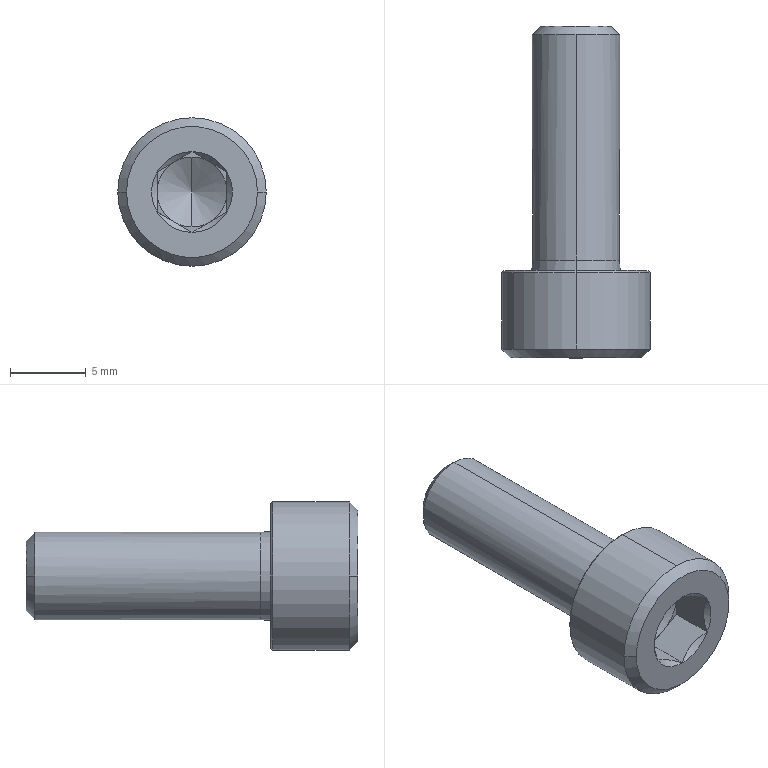Part | SolidWorks | features BaseBody 1 | 1 solid | 35 faces | box 9.808 x 21.923 x 9.808 mm | volume 789.355 mm3 | cone 16 | plane 15 | cylinder 4 | commonest cylinder face diameters 5.769 x2 9.808 x2
STEP:
#1=CARTESIAN_POINT('',(256.285,217.203,292.308));
#2=VERTEX_POINT('',#1);
#3=CARTESIAN_POINT('',(253.4,217.203,295.192));
#4=VERTEX_POINT('',#3);
#5=CARTESIAN_POINT('',(253.4,217.203,292.308));
#6=DIRECTION('',(0.,-1.,0.));
#7=DIRECTION('',(0.,0.,-1.));
#8=AXIS2_PLACEMENT_3D('',#5,#6,#7);
#9=CIRCLE('',#8,2.885);
#10=EDGE_CURVE('',#2,#4,#9,.T.);
#11=ORIENTED_EDGE('',*,*,#10,.T.);
#12=CARTESIAN_POINT('',(253.4,202.308,295.192));
#13=VERTEX_POINT('',#12);
#14=CARTESIAN_POINT('',(253.4,217.769,295.192));
#15=DIRECTION('',(0.,-1.,0.));
#16=VECTOR('',#15,1000.);
#17=LINE('',#14,#16);
#18=EDGE_CURVE('',#4,#13,#17,.T.);
#19=ORIENTED_EDGE('',*,*,#18,.T.);
#20=CARTESIAN_POINT('',(253.4,202.308,289.423));
#21=VERTEX_POINT('',#20);
#22=CARTESIAN_POINT('',(253.4,202.308,292.308));
#23=DIRECTION('',(0.,1.,0.));
#24=DIRECTION('',(0.,0.,-1.));
#25=AXIS2_PLACEMENT_3D('',#22,#23,#24);
#26=CIRCLE('',#25,2.885);
#27=EDGE_CURVE('',#13,#21,#26,.T.);
#28=ORIENTED_EDGE('',*,*,#27,.T.);
#29=CARTESIAN_POINT('',(253.4,217.203,289.423));
#30=VERTEX_POINT('',#29);
#31=CARTESIAN_POINT('',(253.4,217.769,289.423));
#32=DIRECTION('',(0.,-1.,0.));
#33=VECTOR('',#32,1000.);
#34=LINE('',#31,#33);
#35=EDGE_CURVE('',#30,#21,#34,.T.);
#36=ORIENTED_EDGE('',*,*,#35,.F.);
#37=CARTESIAN_POINT('',(253.4,217.203,292.308));
#38=DIRECTION('',(0.,-1.,0.));
#39=DIRECTION('',(0.,0.,-1.));
#40=AXIS2_PLACEMENT_3D('',#37,#38,#39);
#41=CIRCLE('',#40,2.885);
#42=EDGE_CURVE('',#30,#2,#41,.T.);
#43=ORIENTED_EDGE('',*,*,#42,.T.);
#44=EDGE_LOOP('',(#11,#19,#28,#36,#43));
#45=FACE_OUTER_BOUND('',#44,.T.);
#46=CARTESIAN_POINT('',(253.4,217.769,292.308));
#47=DIRECTION('',(0.,-1.,0.));
#48=DIRECTION('',(0.,0.,-1.));
#49=AXIS2_PLACEMENT_3D('',#46,#47,#48);
#50=CYLINDRICAL_SURFACE('',#49,2.885);
#51=ADVANCED_FACE('',(#45),#50,.T.);
#52=CARTESIAN_POINT('',(255.719,217.769,292.308));
#53=VERTEX_POINT('',#52);
#54=CARTESIAN_POINT('',(251.082,217.769,292.308));
#55=VERTEX_POINT('',#54);
#56=CARTESIAN_POINT('',(253.4,217.769,292.308));
#57=DIRECTION('',(0.,-1.,0.));
#58=DIRECTION('',(1.,0.,0.));
#59=AXIS2_PLACEMENT_3D('',#56,#57,#58);
#60=CIRCLE('',#59,2.319);
#61=EDGE_CURVE('',#53,#55,#60,.T.);
#62=ORIENTED_EDGE('',*,*,#61,.T.);
#63=CARTESIAN_POINT('',(250.516,217.203,292.308));
#64=VERTEX_POINT('',#63);
#65=CARTESIAN_POINT('',(250.516,217.203,292.308));
#66=DIRECTION('',(-0.7071,-0.7071,0.));
#67=VECTOR('',#66,1000.);
#68=LINE('',#65,#67);
#69=EDGE_CURVE('',#55,#64,#68,.T.);
#70=ORIENTED_EDGE('',*,*,#69,.T.);
#71=CARTESIAN_POINT('',(253.4,217.203,292.308));
#72=DIRECTION('',(0.,-1.,0.));
#73=DIRECTION('',(0.,0.,-1.));
#74=AXIS2_PLACEMENT_3D('',#71,#72,#73);
#75=CIRCLE('',#74,2.885);
#76=EDGE_CURVE('',#4,#64,#75,.T.);
#77=ORIENTED_EDGE('',*,*,#76,.F.);
#78=ORIENTED_EDGE('',*,*,#10,.F.);
#79=CARTESIAN_POINT('',(256.285,217.203,292.308));
#80=DIRECTION('',(0.7071,-0.7071,0.));
#81=VECTOR('',#80,1000.);
#82=LINE('',#79,#81);
#83=EDGE_CURVE('',#53,#2,#82,.T.);
#84=ORIENTED_EDGE('',*,*,#83,.F.);
#85=EDGE_LOOP('',(#62,#70,#77,#78,#84));
#86=FACE_OUTER_BOUND('',#85,.T.);
#87=CARTESIAN_POINT('',(253.4,217.203,292.308));
#88=DIRECTION('',(0.,-1.,0.));
#89=DIRECTION('',(1.,0.,0.));
#90=AXIS2_PLACEMENT_3D('',#87,#88,#89);
#91=CONICAL_SURFACE('',#90,2.885,0.7854);
#92=ADVANCED_FACE('',(#86),#91,.T.);
#93=ORIENTED_EDGE('',*,*,#27,.F.);
#94=CARTESIAN_POINT('',(253.4,201.615,295.25));
#95=VERTEX_POINT('',#94);
#96=CARTESIAN_POINT('',(253.4,201.615,295.25));
#97=DIRECTION('',(0.,-0.9965,0.08305));
#98=VECTOR('',#97,1000.);
#99=LINE('',#96,#98);
#100=EDGE_CURVE('',#13,#95,#99,.T.);
#101=ORIENTED_EDGE('',*,*,#100,.T.);
#102=CARTESIAN_POINT('',(253.4,201.615,289.365));
#103=VERTEX_POINT('',#102);
#104=CARTESIAN_POINT('',(253.4,201.615,292.308));
#105=DIRECTION('',(0.,1.,0.));
#106=DIRECTION('',(0.,0.,-1.));
#107=AXIS2_PLACEMENT_3D('',#104,#105,#106);
#108=CIRCLE('',#107,2.942);
#109=EDGE_CURVE('',#95,#103,#108,.T.);
#110=ORIENTED_EDGE('',*,*,#109,.T.);
#111=CARTESIAN_POINT('',(253.4,201.615,289.365));
#112=DIRECTION('',(0.,-0.9965,-0.08305));
#113=VECTOR('',#112,1000.);
#114=LINE('',#111,#113);
#115=EDGE_CURVE('',#21,#103,#114,.T.);
#116=ORIENTED_EDGE('',*,*,#115,.F.);
#117=EDGE_LOOP('',(#93,#101,#110,#116));
#118=FACE_OUTER_BOUND('',#117,.T.);
#119=CARTESIAN_POINT('',(253.4,201.615,292.308));
#120=DIRECTION('',(0.,-1.,0.));
#121=DIRECTION('',(0.,0.,-1.));
#122=AXIS2_PLACEMENT_3D('',#119,#120,#121);
#123=CONICAL_SURFACE('',#122,2.942,0.08314);
#124=ADVANCED_FACE('',(#118),#123,.T.);
#125=CARTESIAN_POINT('',(253.4,201.615,287.548));
#126=VERTEX_POINT('',#125);
#127=CARTESIAN_POINT('',(253.4,201.615,297.067));
#128=VERTEX_POINT('',#127);
#129=CARTESIAN_POINT('',(253.4,201.615,292.308));
#130=DIRECTION('',(0.,-1.,0.));
#131=DIRECTION('',(0.,0.,-1.));
#132=AXIS2_PLACEMENT_3D('',#129,#130,#131);
#133=CIRCLE('',#132,4.76);
#134=EDGE_CURVE('',#126,#128,#133,.T.);
#135=ORIENTED_EDGE('',*,*,#134,.T.);
#136=CARTESIAN_POINT('',(253.4,201.471,297.212));
#137=VERTEX_POINT('',#136);
#138=CARTESIAN_POINT('',(253.4,201.471,297.212));
#139=DIRECTION('',(0.,-0.7071,0.7071));
#140=VECTOR('',#139,1000.);
#141=LINE('',#138,#140);
#142=EDGE_CURVE('',#128,#137,#141,.T.);
#143=ORIENTED_EDGE('',*,*,#142,.T.);
#144=CARTESIAN_POINT('',(253.4,201.471,287.404));
#145=VERTEX_POINT('',#144);
#146=CARTESIAN_POINT('',(253.4,201.471,292.308));
#147=DIRECTION('',(0.,1.,0.));
#148=DIRECTION('',(-1.,0.,0.));
#149=AXIS2_PLACEMENT_3D('',#146,#147,#148);
#150=CIRCLE('',#149,4.904);
#151=EDGE_CURVE('',#137,#145,#150,.T.);
#152=ORIENTED_EDGE('',*,*,#151,.T.);
#153=CARTESIAN_POINT('',(253.4,201.471,287.404));
#154=DIRECTION('',(0.,-0.7071,-0.7071));
#155=VECTOR('',#154,1000.);
#156=LINE('',#153,#155);
#157=EDGE_CURVE('',#126,#145,#156,.T.);
#158=ORIENTED_EDGE('',*,*,#157,.F.);
#159=EDGE_LOOP('',(#135,#143,#152,#158));
#160=FACE_OUTER_BOUND('',#159,.T.);
#161=CARTESIAN_POINT('',(253.4,201.471,292.308));
#162=DIRECTION('',(0.,-1.,0.));
#163=DIRECTION('',(0.,0.,-1.));
#164=AXIS2_PLACEMENT_3D('',#161,#162,#163);
#165=CONICAL_SURFACE('',#164,4.904,0.7854);
#166=ADVANCED_FACE('',(#160),#165,.T.);
#167=ORIENTED_EDGE('',*,*,#151,.F.);
#168=CARTESIAN_POINT('',(253.4,196.423,297.212));
#169=VERTEX_POINT('',#168);
#170=CARTESIAN_POINT('',(253.4,217.769,297.212));
#171=DIRECTION('',(0.,-1.,0.));
#172=VECTOR('',#171,1000.);
#173=LINE('',#170,#172);
#174=EDGE_CURVE('',#137,#169,#173,.T.);
#175=ORIENTED_EDGE('',*,*,#174,.T.);
#176=CARTESIAN_POINT('',(258.304,196.423,292.308));
#177=VERTEX_POINT('',#176);
#178=CARTESIAN_POINT('',(253.4,196.423,292.308));
#179=DIRECTION('',(0.,1.,0.));
#180=DIRECTION('',(0.,0.,-1.));
#181=AXIS2_PLACEMENT_3D('',#178,#179,#180);
#182=CIRCLE('',#181,4.904);
#183=EDGE_CURVE('',#169,#177,#182,.T.);
#184=ORIENTED_EDGE('',*,*,#183,.T.);
#185=CARTESIAN_POINT('',(253.4,196.423,287.404));
#186=VERTEX_POINT('',#185);
#187=CARTESIAN_POINT('',(253.4,196.423,292.308));
#188=DIRECTION('',(0.,1.,0.));
#189=DIRECTION('',(0.,0.,-1.));
#190=AXIS2_PLACEMENT_3D('',#187,#188,#189);
#191=CIRCLE('',#190,4.904);
#192=EDGE_CURVE('',#177,#186,#191,.T.);
#193=ORIENTED_EDGE('',*,*,#192,.T.);
#194=CARTESIAN_POINT('',(253.4,217.769,287.404));
#195=DIRECTION('',(0.,-1.,0.));
#196=VECTOR('',#195,1000.);
#197=LINE('',#194,#196);
#198=EDGE_CURVE('',#145,#186,#197,.T.);
#199=ORIENTED_EDGE('',*,*,#198,.F.);
#200=EDGE_LOOP('',(#167,#175,#184,#193,#199));
#201=FACE_OUTER_BOUND('',#200,.T.);
#202=CARTESIAN_POINT('',(253.4,217.769,292.308));
#203=DIRECTION('',(0.,-1.,0.));
#204=DIRECTION('',(0.,0.,-1.));
#205=AXIS2_PLACEMENT_3D('',#202,#203,#204);
#206=CYLINDRICAL_SURFACE('',#205,4.904);
#207=ADVANCED_FACE('',(#201),#206,.T.);
#208=CARTESIAN_POINT('',(249.073,195.846,292.308));
#209=VERTEX_POINT('',#208);
#210=CARTESIAN_POINT('',(257.727,195.846,292.308));
#211=VERTEX_POINT('',#210);
#212=CARTESIAN_POINT('',(253.4,195.846,292.308));
#213=DIRECTION('',(0.,1.,0.));
#214=DIRECTION('',(-1.,0.,0.));
#215=AXIS2_PLACEMENT_3D('',#212,#213,#214);
#216=CIRCLE('',#215,4.327);
#217=EDGE_CURVE('',#209,#211,#216,.T.);
#218=ORIENTED_EDGE('',*,*,#217,.T.);
#219=CARTESIAN_POINT('',(258.304,196.423,292.308));
#220=DIRECTION('',(0.7071,0.7071,0.));
#221=VECTOR('',#220,1000.);
#222=LINE('',#219,#221);
#223=EDGE_CURVE('',#211,#177,#222,.T.);
#224=ORIENTED_EDGE('',*,*,#223,.T.);
#225=ORIENTED_EDGE('',*,*,#183,.F.);
#226=CARTESIAN_POINT('',(248.497,196.423,292.308));
#227=VERTEX_POINT('',#226);
#228=CARTESIAN_POINT('',(253.4,196.423,292.308));
#229=DIRECTION('',(0.,1.,0.));
#230=DIRECTION('',(0.,0.,-1.));
#231=AXIS2_PLACEMENT_3D('',#228,#229,#230);
#232=CIRCLE('',#231,4.904);
#233=EDGE_CURVE('',#227,#169,#232,.T.);
#234=ORIENTED_EDGE('',*,*,#233,.F.);
#235=CARTESIAN_POINT('',(248.497,196.423,292.308));
#236=DIRECTION('',(-0.7071,0.7071,0.));
#237=VECTOR('',#236,1000.);
#238=LINE('',#235,#237);
#239=EDGE_CURVE('',#209,#227,#238,.T.);
#240=ORIENTED_EDGE('',*,*,#239,.F.);
#241=EDGE_LOOP('',(#218,#224,#225,#234,#240));
#242=FACE_OUTER_BOUND('',#241,.T.);
#243=CARTESIAN_POINT('',(253.4,196.423,292.308));
#244=DIRECTION('',(0.,1.,0.));
#245=DIRECTION('',(-1.,0.,0.));
#246=AXIS2_PLACEMENT_3D('',#243,#244,#245);
#247=CONICAL_SURFACE('',#246,4.904,0.7854);
#248=ADVANCED_FACE('',(#242),#247,.T.);
#249=CARTESIAN_POINT('',(253.4,200.063,292.308));
#250=VERTEX_POINT('',#249);
#251=CARTESIAN_POINT('',(253.4,198.731,290.));
#252=VERTEX_POINT('',#251);
#253=CARTESIAN_POINT('',(253.4,198.731,290.));
#254=DIRECTION('',(0.,-0.5,-0.866));
#255=VECTOR('',#254,1000.);
#256=LINE('',#253,#255);
#257=EDGE_CURVE('',#250,#252,#256,.T.);
#258=ORIENTED_EDGE('',*,*,#257,.F.);
#259=CARTESIAN_POINT('',(253.4,198.731,294.615));
#260=VERTEX_POINT('',#259);
#261=CARTESIAN_POINT('',(253.4,198.731,294.615));
#262=DIRECTION('',(0.,-0.5,0.866));
#263=VECTOR('',#262,1000.);
#264=LINE('',#261,#263);
#265=EDGE_CURVE('',#250,#260,#264,.T.);
#266=ORIENTED_EDGE('',*,*,#265,.T.);
#267=CARTESIAN_POINT('',(252.247,198.731,294.306));
#268=VERTEX_POINT('',#267);
#269=CARTESIAN_POINT('',(253.4,198.731,292.308));
#270=DIRECTION('',(0.,1.,0.));
#271=DIRECTION('',(0.,0.,-1.));
#272=AXIS2_PLACEMENT_3D('',#269,#270,#271);
#273=CIRCLE('',#272,2.308);
#274=EDGE_CURVE('',#268,#260,#273,.T.);
#275=ORIENTED_EDGE('',*,*,#274,.F.);
#276=CARTESIAN_POINT('',(251.093,198.731,292.308));
#277=VERTEX_POINT('',#276);
#278=CARTESIAN_POINT('',(253.4,198.731,292.308));
#279=DIRECTION('',(0.,1.,0.));
#280=DIRECTION('',(0.,0.,-1.));
#281=AXIS2_PLACEMENT_3D('',#278,#279,#280);
#282=CIRCLE('',#281,2.308);
#283=EDGE_CURVE('',#277,#268,#282,.T.);
#284=ORIENTED_EDGE('',*,*,#283,.F.);
#285=CARTESIAN_POINT('',(252.247,198.731,290.309));
#286=VERTEX_POINT('',#285);
#287=CARTESIAN_POINT('',(253.4,198.731,292.308));
#288=DIRECTION('',(0.,1.,0.));
#289=DIRECTION('',(0.,0.,-1.));
#290=AXIS2_PLACEMENT_3D('',#287,#288,#289);
#291=CIRCLE('',#290,2.308);
#292=EDGE_CURVE('',#286,#277,#291,.T.);
#293=ORIENTED_EDGE('',*,*,#292,.F.);
#294=CARTESIAN_POINT('',(253.4,198.731,292.308));
#295=DIRECTION('',(0.,1.,0.));
#296=DIRECTION('',(0.,0.,-1.));
#297=AXIS2_PLACEMENT_3D('',#294,#295,#296);
#298=CIRCLE('',#297,2.308);
#299=EDGE_CURVE('',#252,#286,#298,.T.);
#300=ORIENTED_EDGE('',*,*,#299,.F.);
#301=EDGE_LOOP('',(#258,#266,#275,#284,#293,#300));
#302=FACE_OUTER_BOUND('',#301,.T.);
#303=CARTESIAN_POINT('',(253.4,198.731,292.308));
#304=DIRECTION('',(0.,-1.,0.));
#305=DIRECTION('',(0.,0.,-1.));
#306=AXIS2_PLACEMENT_3D('',#303,#304,#305);
#307=CONICAL_SURFACE('',#306,2.308,1.047);
#308=ADVANCED_FACE('',(#302),#307,.F.);
#309=ORIENTED_EDGE('',*,*,#18,.F.);
#310=ORIENTED_EDGE('',*,*,#76,.T.);
#311=CARTESIAN_POINT('',(253.4,217.203,292.308));
#312=DIRECTION('',(0.,-1.,0.));
#313=DIRECTION('',(0.,0.,-1.));
#314=AXIS2_PLACEMENT_3D('',#311,#312,#313);
#315=CIRCLE('',#314,2.885);
#316=EDGE_CURVE('',#64,#30,#315,.T.);
#317=ORIENTED_EDGE('',*,*,#316,.T.);
#318=ORIENTED_EDGE('',*,*,#35,.T.);
#319=CARTESIAN_POINT('',(253.4,202.308,292.308));
#320=DIRECTION('',(0.,1.,0.));
#321=DIRECTION('',(0.,0.,-1.));
#322=AXIS2_PLACEMENT_3D('',#319,#320,#321);
#323=CIRCLE('',#322,2.885);
#324=EDGE_CURVE('',#21,#13,#323,.T.);
#325=ORIENTED_EDGE('',*,*,#324,.T.);
#326=EDGE_LOOP('',(#309,#310,#317,#318,#325));
#327=FACE_OUTER_BOUND('',#326,.T.);
#328=CARTESIAN_POINT('',(253.4,217.769,292.308));
#329=DIRECTION('',(0.,-1.,0.));
#330=DIRECTION('',(0.,0.,-1.));
#331=AXIS2_PLACEMENT_3D('',#328,#329,#330);
#332=CYLINDRICAL_SURFACE('',#331,2.885);
#333=ADVANCED_FACE('',(#327),#332,.T.);
#334=ORIENTED_EDGE('',*,*,#69,.F.);
#335=CARTESIAN_POINT('',(253.4,217.769,292.308));
#336=DIRECTION('',(0.,-1.,0.));
#337=DIRECTION('',(1.,0.,0.));
#338=AXIS2_PLACEMENT_3D('',#335,#336,#337);
#339=CIRCLE('',#338,2.319);
#340=EDGE_CURVE('',#55,#53,#339,.T.);
#341=ORIENTED_EDGE('',*,*,#340,.T.);
#342=ORIENTED_EDGE('',*,*,#83,.T.);
#343=ORIENTED_EDGE('',*,*,#42,.F.);
#344=ORIENTED_EDGE('',*,*,#316,.F.);
#345=EDGE_LOOP('',(#334,#341,#342,#343,#344));
#346=FACE_OUTER_BOUND('',#345,.T.);
#347=CARTESIAN_POINT('',(253.4,217.203,292.308));
#348=DIRECTION('',(0.,-1.,0.));
#349=DIRECTION('',(1.,0.,0.));
#350=AXIS2_PLACEMENT_3D('',#347,#348,#349);
#351=CONICAL_SURFACE('',#350,2.885,0.7854);
#352=ADVANCED_FACE('',(#346),#351,.T.);
#353=ORIENTED_EDGE('',*,*,#100,.F.);
#354=ORIENTED_EDGE('',*,*,#324,.F.);
#355=ORIENTED_EDGE('',*,*,#115,.T.);
#356=CARTESIAN_POINT('',(253.4,201.615,292.308));
#357=DIRECTION('',(0.,1.,0.));
#358=DIRECTION('',(0.,0.,-1.));
#359=AXIS2_PLACEMENT_3D('',#356,#357,#358);
#360=CIRCLE('',#359,2.942);
#361=EDGE_CURVE('',#103,#95,#360,.T.);
#362=ORIENTED_EDGE('',*,*,#361,.T.);
#363=EDGE_LOOP('',(#353,#354,#355,#362));
#364=FACE_OUTER_BOUND('',#363,.T.);
#365=CARTESIAN_POINT('',(253.4,201.615,292.308));
#366=DIRECTION('',(0.,-1.,0.));
#367=DIRECTION('',(0.,0.,-1.));
#368=AXIS2_PLACEMENT_3D('',#365,#366,#367);
#369=CONICAL_SURFACE('',#368,2.942,0.08314);
#370=ADVANCED_FACE('',(#364),#369,.T.);
#371=ORIENTED_EDGE('',*,*,#61,.F.);
#372=ORIENTED_EDGE('',*,*,#340,.F.);
#373=EDGE_LOOP('',(#371,#372));
#374=FACE_OUTER_BOUND('',#373,.T.);
#375=CARTESIAN_POINT('',(251.082,217.769,292.308));
#376=DIRECTION('',(0.,-1.,0.));
#377=DIRECTION('',(0.,0.,-1.));
#378=AXIS2_PLACEMENT_3D('',#375,#376,#377);
#379=PLANE('',#378);
#380=ADVANCED_FACE('',(#374),#379,.F.);
#381=ORIENTED_EDGE('',*,*,#361,.F.);
#382=ORIENTED_EDGE('',*,*,#109,.F.);
#383=EDGE_LOOP('',(#381,#382));
#384=FACE_BOUND('',#383,.T.);
#385=ORIENTED_EDGE('',*,*,#134,.F.);
#386=CARTESIAN_POINT('',(253.4,201.615,292.308));
#387=DIRECTION('',(0.,-1.,0.));
#388=DIRECTION('',(0.,0.,-1.));
#389=AXIS2_PLACEMENT_3D('',#386,#387,#388);
#390=CIRCLE('',#389,4.76);
#391=EDGE_CURVE('',#128,#126,#390,.T.);
#392=ORIENTED_EDGE('',*,*,#391,.F.);
#393=EDGE_LOOP('',(#385,#392));
#394=FACE_OUTER_BOUND('',#393,.T.);
#395=CARTESIAN_POINT('',(248.641,201.615,292.308));
#396=DIRECTION('',(0.,-1.,0.));
#397=DIRECTION('',(0.,0.,-1.));
#398=AXIS2_PLACEMENT_3D('',#395,#396,#397);
#399=PLANE('',#398);
#400=ADVANCED_FACE('',(#384,#394),#399,.F.);
#401=ORIENTED_EDGE('',*,*,#142,.F.);
#402=ORIENTED_EDGE('',*,*,#391,.T.);
#403=ORIENTED_EDGE('',*,*,#157,.T.);
#404=CARTESIAN_POINT('',(253.4,201.471,292.308));
#405=DIRECTION('',(0.,1.,0.));
#406=DIRECTION('',(-1.,0.,0.));
#407=AXIS2_PLACEMENT_3D('',#404,#405,#406);
#408=CIRCLE('',#407,4.904);
#409=EDGE_CURVE('',#145,#137,#408,.T.);
#410=ORIENTED_EDGE('',*,*,#409,.T.);
#411=EDGE_LOOP('',(#401,#402,#403,#410));
#412=FACE_OUTER_BOUND('',#411,.T.);
#413=CARTESIAN_POINT('',(253.4,201.471,292.308));
#414=DIRECTION('',(0.,-1.,0.));
#415=DIRECTION('',(0.,0.,-1.));
#416=AXIS2_PLACEMENT_3D('',#413,#414,#415);
#417=CONICAL_SURFACE('',#416,4.904,0.7854);
#418=ADVANCED_FACE('',(#412),#417,.T.);
#419=ORIENTED_EDGE('',*,*,#174,.F.);
#420=ORIENTED_EDGE('',*,*,#409,.F.);
#421=ORIENTED_EDGE('',*,*,#198,.T.);
#422=CARTESIAN_POINT('',(253.4,196.423,292.308));
#423=DIRECTION('',(0.,1.,0.));
#424=DIRECTION('',(0.,0.,-1.));
#425=AXIS2_PLACEMENT_3D('',#422,#423,#424);
#426=CIRCLE('',#425,4.904);
#427=EDGE_CURVE('',#186,#227,#426,.T.);
#428=ORIENTED_EDGE('',*,*,#427,.T.);
#429=ORIENTED_EDGE('',*,*,#233,.T.);
#430=EDGE_LOOP('',(#419,#420,#421,#428,#429));
#431=FACE_OUTER_BOUND('',#430,.T.);
#432=CARTESIAN_POINT('',(253.4,217.769,292.308));
#433=DIRECTION('',(0.,-1.,0.));
#434=DIRECTION('',(0.,0.,-1.));
#435=AXIS2_PLACEMENT_3D('',#432,#433,#434);
#436=CYLINDRICAL_SURFACE('',#435,4.904);
#437=ADVANCED_FACE('',(#431),#436,.T.);
#438=ORIENTED_EDGE('',*,*,#223,.F.);
#439=CARTESIAN_POINT('',(253.4,195.846,292.308));
#440=DIRECTION('',(0.,1.,0.));
#441=DIRECTION('',(-1.,0.,0.));
#442=AXIS2_PLACEMENT_3D('',#439,#440,#441);
#443=CIRCLE('',#442,4.327);
#444=EDGE_CURVE('',#211,#209,#443,.T.);
#445=ORIENTED_EDGE('',*,*,#444,.T.);
#446=ORIENTED_EDGE('',*,*,#239,.T.);
#447=ORIENTED_EDGE('',*,*,#427,.F.);
#448=ORIENTED_EDGE('',*,*,#192,.F.);
#449=EDGE_LOOP('',(#438,#445,#446,#447,#448));
#450=FACE_OUTER_BOUND('',#449,.T.);
#451=CARTESIAN_POINT('',(253.4,196.423,292.308));
#452=DIRECTION('',(0.,1.,0.));
#453=DIRECTION('',(-1.,0.,0.));
#454=AXIS2_PLACEMENT_3D('',#451,#452,#453);
#455=CONICAL_SURFACE('',#454,4.904,0.7854);
#456=ADVANCED_FACE('',(#450),#455,.T.);
#457=CARTESIAN_POINT('',(255.708,195.846,293.64));
#458=VERTEX_POINT('',#457);
#459=CARTESIAN_POINT('',(253.4,195.846,294.972));
#460=VERTEX_POINT('',#459);
#461=CARTESIAN_POINT('',(253.4,195.846,292.308));
#462=DIRECTION('',(0.,-1.,0.));
#463=DIRECTION('',(1.,0.,0.));
#464=AXIS2_PLACEMENT_3D('',#461,#462,#463);
#465=CIRCLE('',#464,2.665);
#466=EDGE_CURVE('',#458,#460,#465,.T.);
#467=ORIENTED_EDGE('',*,*,#466,.F.);
#468=CARTESIAN_POINT('',(255.708,195.846,290.975));
#469=VERTEX_POINT('',#468);
#470=CARTESIAN_POINT('',(253.4,195.846,292.308));
#471=DIRECTION('',(0.,-1.,0.));
#472=DIRECTION('',(0.,0.,-1.));
#473=AXIS2_PLACEMENT_3D('',#470,#471,#472);
#474=CIRCLE('',#473,2.665);
#475=EDGE_CURVE('',#469,#458,#474,.T.);
#476=ORIENTED_EDGE('',*,*,#475,.F.);
#477=CARTESIAN_POINT('',(253.4,195.846,289.643));
#478=VERTEX_POINT('',#477);
#479=CARTESIAN_POINT('',(253.4,195.846,292.308));
#480=DIRECTION('',(0.,-1.,0.));
#481=DIRECTION('',(0.,0.,-1.));
#482=AXIS2_PLACEMENT_3D('',#479,#480,#481);
#483=CIRCLE('',#482,2.665);
#484=EDGE_CURVE('',#478,#469,#483,.T.);
#485=ORIENTED_EDGE('',*,*,#484,.F.);
#486=CARTESIAN_POINT('',(251.093,195.846,290.975));
#487=VERTEX_POINT('',#486);
#488=CARTESIAN_POINT('',(253.4,195.846,292.308));
#489=DIRECTION('',(0.,-1.,0.));
#490=DIRECTION('',(0.,0.,-1.));
#491=AXIS2_PLACEMENT_3D('',#488,#489,#490);
#492=CIRCLE('',#491,2.665);
#493=EDGE_CURVE('',#487,#478,#492,.T.);
#494=ORIENTED_EDGE('',*,*,#493,.F.);
#495=CARTESIAN_POINT('',(251.093,195.846,293.64));
#496=VERTEX_POINT('',#495);
#497=CARTESIAN_POINT('',(253.4,195.846,292.308));
#498=DIRECTION('',(0.,-1.,0.));
#499=DIRECTION('',(0.,0.,-1.));
#500=AXIS2_PLACEMENT_3D('',#497,#498,#499);
#501=CIRCLE('',#500,2.665);
#502=EDGE_CURVE('',#496,#487,#501,.T.);
#503=ORIENTED_EDGE('',*,*,#502,.F.);
#504=CARTESIAN_POINT('',(253.4,195.846,292.308));
#505=DIRECTION('',(0.,-1.,0.));
#506=DIRECTION('',(0.,0.,-1.));
#507=AXIS2_PLACEMENT_3D('',#504,#505,#506);
#508=CIRCLE('',#507,2.665);
#509=EDGE_CURVE('',#460,#496,#508,.T.);
#510=ORIENTED_EDGE('',*,*,#509,.F.);
#511=EDGE_LOOP('',(#467,#476,#485,#494,#503,#510));
#512=FACE_BOUND('',#511,.T.);
#513=ORIENTED_EDGE('',*,*,#217,.F.);
#514=ORIENTED_EDGE('',*,*,#444,.F.);
#515=EDGE_LOOP('',(#513,#514));
#516=FACE_OUTER_BOUND('',#515,.T.);
#517=CARTESIAN_POINT('',(250.736,195.846,292.308));
#518=DIRECTION('',(0.,1.,0.));
#519=DIRECTION('',(0.,0.,1.));
#520=AXIS2_PLACEMENT_3D('',#517,#518,#519);
#521=PLANE('',#520);
#522=ADVANCED_FACE('',(#512,#516),#521,.F.);
#523=CARTESIAN_POINT('',(253.4,195.846,294.972));
#524=CARTESIAN_POINT('',(253.22,195.95,294.868));
#525=CARTESIAN_POINT('',(253.036,196.039,294.762));
#526=CARTESIAN_POINT('',(252.749,196.134,294.596));
#527=CARTESIAN_POINT('',(252.652,196.159,294.54));
#528=CARTESIAN_POINT('',(252.454,196.194,294.426));
#529=CARTESIAN_POINT('',(252.352,196.203,294.367));
#530=CARTESIAN_POINT('',(252.049,196.204,294.192));
#531=CARTESIAN_POINT('',(251.851,196.168,294.078));
#532=CARTESIAN_POINT('',(251.461,196.041,293.853));
#533=CARTESIAN_POINT('',(251.274,195.951,293.745));
#534=CARTESIAN_POINT('',(251.093,195.846,293.64));
#535=B_SPLINE_CURVE_WITH_KNOTS('',3,(#523,#524,#525,#526,#527,#528,#529,#530,#531,#532,#533,#534),.UNSPECIFIED.,.F.,.F.,(4,2,2,2,2,4),(0.,0.0006881,0.001032,0.001376,0.002064,0.002753),.UNSPECIFIED.);
#536=EDGE_CURVE('',#460,#496,#535,.T.);
#537=ORIENTED_EDGE('',*,*,#536,.F.);
#538=ORIENTED_EDGE('',*,*,#509,.T.);
#539=EDGE_LOOP('',(#537,#538));
#540=FACE_OUTER_BOUND('',#539,.T.);
#541=CARTESIAN_POINT('',(253.4,195.846,292.308));
#542=DIRECTION('',(0.,-1.,0.));
#543=DIRECTION('',(0.,0.,-1.));
#544=AXIS2_PLACEMENT_3D('',#541,#542,#543);
#545=CONICAL_SURFACE('',#544,2.665,0.7854);
#546=ADVANCED_FACE('',(#540),#545,.F.);
#547=CARTESIAN_POINT('',(255.708,195.846,293.64));
#548=CARTESIAN_POINT('',(255.528,195.95,293.744));
#549=CARTESIAN_POINT('',(255.343,196.039,293.851));
#550=CARTESIAN_POINT('',(255.057,196.134,294.016));
#551=CARTESIAN_POINT('',(254.96,196.159,294.072));
#552=CARTESIAN_POINT('',(254.761,196.194,294.187));
#553=CARTESIAN_POINT('',(254.659,196.203,294.246));
#554=CARTESIAN_POINT('',(254.357,196.204,294.42));
#555=CARTESIAN_POINT('',(254.159,196.168,294.534));
#556=CARTESIAN_POINT('',(253.768,196.041,294.76));
#557=CARTESIAN_POINT('',(253.582,195.951,294.868));
#558=CARTESIAN_POINT('',(253.4,195.846,294.972));
#559=B_SPLINE_CURVE_WITH_KNOTS('',3,(#547,#548,#549,#550,#551,#552,#553,#554,#555,#556,#557,#558),.UNSPECIFIED.,.F.,.F.,(4,2,2,2,2,4),(0.,0.0006881,0.001032,0.001376,0.002064,0.002753),.UNSPECIFIED.);
#560=EDGE_CURVE('',#458,#460,#559,.T.);
#561=ORIENTED_EDGE('',*,*,#560,.F.);
#562=ORIENTED_EDGE('',*,*,#466,.T.);
#563=EDGE_LOOP('',(#561,#562));
#564=FACE_OUTER_BOUND('',#563,.T.);
#565=CARTESIAN_POINT('',(253.4,195.846,292.308));
#566=DIRECTION('',(0.,-1.,0.));
#567=DIRECTION('',(1.,0.,0.));
#568=AXIS2_PLACEMENT_3D('',#565,#566,#567);
#569=CONICAL_SURFACE('',#568,2.665,0.7854);
#570=ADVANCED_FACE('',(#564),#569,.F.);
#571=CARTESIAN_POINT('',(255.708,195.846,290.975));
#572=CARTESIAN_POINT('',(255.708,195.95,291.184));
#573=CARTESIAN_POINT('',(255.708,196.039,291.396));
#574=CARTESIAN_POINT('',(255.708,196.134,291.727));
#575=CARTESIAN_POINT('',(255.708,196.159,291.839));
#576=CARTESIAN_POINT('',(255.708,196.194,292.068));
#577=CARTESIAN_POINT('',(255.708,196.203,292.186));
#578=CARTESIAN_POINT('',(255.708,196.204,292.535));
#579=CARTESIAN_POINT('',(255.708,196.168,292.764));
#580=CARTESIAN_POINT('',(255.708,196.041,293.215));
#581=CARTESIAN_POINT('',(255.708,195.951,293.431));
#582=CARTESIAN_POINT('',(255.708,195.846,293.64));
#583=B_SPLINE_CURVE_WITH_KNOTS('',3,(#571,#572,#573,#574,#575,#576,#577,#578,#579,#580,#581,#582),.UNSPECIFIED.,.F.,.F.,(4,2,2,2,2,4),(0.,0.0006881,0.001032,0.001376,0.002064,0.002753),.UNSPECIFIED.);
#584=EDGE_CURVE('',#469,#458,#583,.T.);
#585=ORIENTED_EDGE('',*,*,#584,.F.);
#586=ORIENTED_EDGE('',*,*,#475,.T.);
#587=EDGE_LOOP('',(#585,#586));
#588=FACE_OUTER_BOUND('',#587,.T.);
#589=CARTESIAN_POINT('',(253.4,195.846,292.308));
#590=DIRECTION('',(0.,-1.,0.));
#591=DIRECTION('',(0.,0.,-1.));
#592=AXIS2_PLACEMENT_3D('',#589,#590,#591);
#593=CONICAL_SURFACE('',#592,2.665,0.7854);
#594=ADVANCED_FACE('',(#588),#593,.F.);
#595=CARTESIAN_POINT('',(253.4,195.846,289.643));
#596=CARTESIAN_POINT('',(253.581,195.95,289.747));
#597=CARTESIAN_POINT('',(253.765,196.039,289.854));
#598=CARTESIAN_POINT('',(254.052,196.134,290.019));
#599=CARTESIAN_POINT('',(254.149,196.159,290.075));
#600=CARTESIAN_POINT('',(254.347,196.194,290.19));
#601=CARTESIAN_POINT('',(254.449,196.203,290.249));
#602=CARTESIAN_POINT('',(254.751,196.204,290.423));
#603=CARTESIAN_POINT('',(254.949,196.168,290.537));
#604=CARTESIAN_POINT('',(255.34,196.041,290.763));
#605=CARTESIAN_POINT('',(255.527,195.951,290.871));
#606=CARTESIAN_POINT('',(255.708,195.846,290.975));
#607=B_SPLINE_CURVE_WITH_KNOTS('',3,(#595,#596,#597,#598,#599,#600,#601,#602,#603,#604,#605,#606),.UNSPECIFIED.,.F.,.F.,(4,2,2,2,2,4),(0.,0.0006881,0.001032,0.001376,0.002064,0.002753),.UNSPECIFIED.);
#608=EDGE_CURVE('',#478,#469,#607,.T.);
#609=ORIENTED_EDGE('',*,*,#608,.F.);
#610=ORIENTED_EDGE('',*,*,#484,.T.);
#611=EDGE_LOOP('',(#609,#610));
#612=FACE_OUTER_BOUND('',#611,.T.);
#613=CARTESIAN_POINT('',(253.4,195.846,292.308));
#614=DIRECTION('',(0.,-1.,0.));
#615=DIRECTION('',(0.,0.,-1.));
#616=AXIS2_PLACEMENT_3D('',#613,#614,#615);
#617=CONICAL_SURFACE('',#616,2.665,0.7854);
#618=ADVANCED_FACE('',(#612),#617,.F.);
#619=CARTESIAN_POINT('',(251.093,195.846,290.975));
#620=CARTESIAN_POINT('',(251.273,195.95,290.871));
#621=CARTESIAN_POINT('',(251.457,196.039,290.765));
#622=CARTESIAN_POINT('',(251.744,196.134,290.599));
#623=CARTESIAN_POINT('',(251.841,196.159,290.543));
#624=CARTESIAN_POINT('',(252.039,196.194,290.429));
#625=CARTESIAN_POINT('',(252.142,196.203,290.37));
#626=CARTESIAN_POINT('',(252.444,196.204,290.195));
#627=CARTESIAN_POINT('',(252.642,196.168,290.081));
#628=CARTESIAN_POINT('',(253.032,196.041,289.856));
#629=CARTESIAN_POINT('',(253.219,195.951,289.748));
#630=CARTESIAN_POINT('',(253.4,195.846,289.643));
#631=B_SPLINE_CURVE_WITH_KNOTS('',3,(#619,#620,#621,#622,#623,#624,#625,#626,#627,#628,#629,#630),.UNSPECIFIED.,.F.,.F.,(4,2,2,2,2,4),(0.,0.0006881,0.001032,0.001376,0.002064,0.002753),.UNSPECIFIED.);
#632=EDGE_CURVE('',#487,#478,#631,.T.);
#633=ORIENTED_EDGE('',*,*,#632,.F.);
#634=ORIENTED_EDGE('',*,*,#493,.T.);
#635=EDGE_LOOP('',(#633,#634));
#636=FACE_OUTER_BOUND('',#635,.T.);
#637=CARTESIAN_POINT('',(253.4,195.846,292.308));
#638=DIRECTION('',(0.,-1.,0.));
#639=DIRECTION('',(0.,0.,-1.));
#640=AXIS2_PLACEMENT_3D('',#637,#638,#639);
#641=CONICAL_SURFACE('',#640,2.665,0.7854);
#642=ADVANCED_FACE('',(#636),#641,.F.);
#643=CARTESIAN_POINT('',(251.093,195.846,293.64));
#644=CARTESIAN_POINT('',(251.093,195.95,293.432));
#645=CARTESIAN_POINT('',(251.093,196.039,293.219));
#646=CARTESIAN_POINT('',(251.093,196.134,292.888));
#647=CARTESIAN_POINT('',(251.093,196.159,292.776));
#648=CARTESIAN_POINT('',(251.093,196.194,292.547));
#649=CARTESIAN_POINT('',(251.093,196.203,292.429));
#650=CARTESIAN_POINT('',(251.093,196.204,292.08));
#651=CARTESIAN_POINT('',(251.093,196.168,291.851));
#652=CARTESIAN_POINT('',(251.093,196.041,291.4));
#653=CARTESIAN_POINT('',(251.093,195.951,291.185));
#654=CARTESIAN_POINT('',(251.093,195.846,290.975));
#655=B_SPLINE_CURVE_WITH_KNOTS('',3,(#643,#644,#645,#646,#647,#648,#649,#650,#651,#652,#653,#654),.UNSPECIFIED.,.F.,.F.,(4,2,2,2,2,4),(0.,0.0006881,0.001032,0.001376,0.002064,0.002753),.UNSPECIFIED.);
#656=EDGE_CURVE('',#496,#487,#655,.T.);
#657=ORIENTED_EDGE('',*,*,#656,.F.);
#658=ORIENTED_EDGE('',*,*,#502,.T.);
#659=EDGE_LOOP('',(#657,#658));
#660=FACE_OUTER_BOUND('',#659,.T.);
#661=CARTESIAN_POINT('',(253.4,195.846,292.308));
#662=DIRECTION('',(0.,-1.,0.));
#663=DIRECTION('',(0.,0.,-1.));
#664=AXIS2_PLACEMENT_3D('',#661,#662,#663);
#665=CONICAL_SURFACE('',#664,2.665,0.7854);
#666=ADVANCED_FACE('',(#660),#665,.F.);
#667=CARTESIAN_POINT('',(251.093,198.731,293.64));
#668=VERTEX_POINT('',#667);
#669=CARTESIAN_POINT('',(251.093,198.731,293.64));
#670=DIRECTION('',(0.,-1.,0.));
#671=VECTOR('',#670,1000.);
#672=LINE('',#669,#671);
#673=EDGE_CURVE('',#668,#496,#672,.T.);
#674=ORIENTED_EDGE('',*,*,#673,.F.);
#675=CARTESIAN_POINT('',(253.4,198.731,294.972));
#676=DIRECTION('',(-0.866,0.,-0.5));
#677=VECTOR('',#676,1000.);
#678=LINE('',#675,#677);
#679=EDGE_CURVE('',#268,#668,#678,.T.);
#680=ORIENTED_EDGE('',*,*,#679,.F.);
#681=CARTESIAN_POINT('',(253.4,198.731,294.972));
#682=VERTEX_POINT('',#681);
#683=CARTESIAN_POINT('',(253.4,198.731,294.972));
#684=DIRECTION('',(-0.866,0.,-0.5));
#685=VECTOR('',#684,1000.);
#686=LINE('',#683,#685);
#687=EDGE_CURVE('',#682,#268,#686,.T.);
#688=ORIENTED_EDGE('',*,*,#687,.F.);
#689=CARTESIAN_POINT('',(253.4,198.731,294.972));
#690=DIRECTION('',(0.,1.,0.));
#691=VECTOR('',#690,1000.);
#692=LINE('',#689,#691);
#693=EDGE_CURVE('',#460,#682,#692,.T.);
#694=ORIENTED_EDGE('',*,*,#693,.F.);
#695=ORIENTED_EDGE('',*,*,#536,.T.);
#696=EDGE_LOOP('',(#674,#680,#688,#694,#695));
#697=FACE_OUTER_BOUND('',#696,.T.);
#698=CARTESIAN_POINT('',(253.4,198.731,294.972));
#699=DIRECTION('',(-0.5,0.,0.866));
#700=DIRECTION('',(0.866,0.,0.5));
#701=AXIS2_PLACEMENT_3D('',#698,#699,#700);
#702=PLANE('',#701);
#703=ADVANCED_FACE('',(#697),#702,.F.);
#704=ORIENTED_EDGE('',*,*,#693,.T.);
#705=CARTESIAN_POINT('',(254.554,198.731,294.306));
#706=VERTEX_POINT('',#705);
#707=CARTESIAN_POINT('',(255.708,198.731,293.64));
#708=DIRECTION('',(-0.866,0.,0.5));
#709=VECTOR('',#708,1000.);
#710=LINE('',#707,#709);
#711=EDGE_CURVE('',#706,#682,#710,.T.);
#712=ORIENTED_EDGE('',*,*,#711,.F.);
#713=CARTESIAN_POINT('',(255.708,198.731,293.64));
#714=VERTEX_POINT('',#713);
#715=CARTESIAN_POINT('',(255.708,198.731,293.64));
#716=DIRECTION('',(-0.866,0.,0.5));
#717=VECTOR('',#716,1000.);
#718=LINE('',#715,#717);
#719=EDGE_CURVE('',#714,#706,#718,.T.);
#720=ORIENTED_EDGE('',*,*,#719,.F.);
#721=CARTESIAN_POINT('',(255.708,198.731,293.64));
#722=DIRECTION('',(0.,1.,0.));
#723=VECTOR('',#722,1000.);
#724=LINE('',#721,#723);
#725=EDGE_CURVE('',#458,#714,#724,.T.);
#726=ORIENTED_EDGE('',*,*,#725,.F.);
#727=ORIENTED_EDGE('',*,*,#560,.T.);
#728=EDGE_LOOP('',(#704,#712,#720,#726,#727));
#729=FACE_OUTER_BOUND('',#728,.T.);
#730=CARTESIAN_POINT('',(255.708,198.731,293.64));
#731=DIRECTION('',(0.5,0.,0.866));
#732=DIRECTION('',(0.866,0.,-0.5));
#733=AXIS2_PLACEMENT_3D('',#730,#731,#732);
#734=PLANE('',#733);
#735=ADVANCED_FACE('',(#729),#734,.F.);
#736=ORIENTED_EDGE('',*,*,#725,.T.);
#737=CARTESIAN_POINT('',(255.708,198.731,292.308));
#738=VERTEX_POINT('',#737);
#739=CARTESIAN_POINT('',(255.708,198.731,290.975));
#740=DIRECTION('',(0.,0.,1.));
#741=VECTOR('',#740,1000.);
#742=LINE('',#739,#741);
#743=EDGE_CURVE('',#738,#714,#742,.T.);
#744=ORIENTED_EDGE('',*,*,#743,.F.);
#745=CARTESIAN_POINT('',(255.708,198.731,290.975));
#746=VERTEX_POINT('',#745);
#747=CARTESIAN_POINT('',(255.708,198.731,290.975));
#748=DIRECTION('',(0.,0.,1.));
#749=VECTOR('',#748,1000.);
#750=LINE('',#747,#749);
#751=EDGE_CURVE('',#746,#738,#750,.T.);
#752=ORIENTED_EDGE('',*,*,#751,.F.);
#753=CARTESIAN_POINT('',(255.708,198.731,290.975));
#754=DIRECTION('',(0.,1.,0.));
#755=VECTOR('',#754,1000.);
#756=LINE('',#753,#755);
#757=EDGE_CURVE('',#469,#746,#756,.T.);
#758=ORIENTED_EDGE('',*,*,#757,.F.);
#759=ORIENTED_EDGE('',*,*,#584,.T.);
#760=EDGE_LOOP('',(#736,#744,#752,#758,#759));
#761=FACE_OUTER_BOUND('',#760,.T.);
#762=CARTESIAN_POINT('',(255.708,198.731,290.975));
#763=DIRECTION('',(1.,0.,0.));
#764=DIRECTION('',(0.,0.,-1.));
#765=AXIS2_PLACEMENT_3D('',#762,#763,#764);
#766=PLANE('',#765);
#767=ADVANCED_FACE('',(#761),#766,.F.);
#768=ORIENTED_EDGE('',*,*,#757,.T.);
#769=CARTESIAN_POINT('',(254.554,198.731,290.309));
#770=VERTEX_POINT('',#769);
#771=CARTESIAN_POINT('',(253.4,198.731,289.643));
#772=DIRECTION('',(0.866,0.,0.5));
#773=VECTOR('',#772,1000.);
#774=LINE('',#771,#773);
#775=EDGE_CURVE('',#770,#746,#774,.T.);
#776=ORIENTED_EDGE('',*,*,#775,.F.);
#777=CARTESIAN_POINT('',(253.4,198.731,289.643));
#778=VERTEX_POINT('',#777);
#779=CARTESIAN_POINT('',(253.4,198.731,289.643));
#780=DIRECTION('',(0.866,0.,0.5));
#781=VECTOR('',#780,1000.);
#782=LINE('',#779,#781);
#783=EDGE_CURVE('',#778,#770,#782,.T.);
#784=ORIENTED_EDGE('',*,*,#783,.F.);
#785=CARTESIAN_POINT('',(253.4,198.731,289.643));
#786=DIRECTION('',(0.,1.,0.));
#787=VECTOR('',#786,1000.);
#788=LINE('',#785,#787);
#789=EDGE_CURVE('',#478,#778,#788,.T.);
#790=ORIENTED_EDGE('',*,*,#789,.F.);
#791=ORIENTED_EDGE('',*,*,#608,.T.);
#792=EDGE_LOOP('',(#768,#776,#784,#790,#791));
#793=FACE_OUTER_BOUND('',#792,.T.);
#794=CARTESIAN_POINT('',(253.4,198.731,289.643));
#795=DIRECTION('',(0.5,0.,-0.866));
#796=DIRECTION('',(-0.866,0.,-0.5));
#797=AXIS2_PLACEMENT_3D('',#794,#795,#796);
#798=PLANE('',#797);
#799=ADVANCED_FACE('',(#793),#798,.F.);
#800=ORIENTED_EDGE('',*,*,#789,.T.);
#801=CARTESIAN_POINT('',(251.093,198.731,290.975));
#802=DIRECTION('',(0.866,0.,-0.5));
#803=VECTOR('',#802,1000.);
#804=LINE('',#801,#803);
#805=EDGE_CURVE('',#286,#778,#804,.T.);
#806=ORIENTED_EDGE('',*,*,#805,.F.);
#807=CARTESIAN_POINT('',(251.093,198.731,290.975));
#808=VERTEX_POINT('',#807);
#809=CARTESIAN_POINT('',(251.093,198.731,290.975));
#810=DIRECTION('',(0.866,0.,-0.5));
#811=VECTOR('',#810,1000.);
#812=LINE('',#809,#811);
#813=EDGE_CURVE('',#808,#286,#812,.T.);
#814=ORIENTED_EDGE('',*,*,#813,.F.);
#815=CARTESIAN_POINT('',(251.093,198.731,290.975));
#816=DIRECTION('',(0.,1.,0.));
#817=VECTOR('',#816,1000.);
#818=LINE('',#815,#817);
#819=EDGE_CURVE('',#487,#808,#818,.T.);
#820=ORIENTED_EDGE('',*,*,#819,.F.);
#821=ORIENTED_EDGE('',*,*,#632,.T.);
#822=EDGE_LOOP('',(#800,#806,#814,#820,#821));
#823=FACE_OUTER_BOUND('',#822,.T.);
#824=CARTESIAN_POINT('',(251.093,198.731,290.975));
#825=DIRECTION('',(-0.5,0.,-0.866));
#826=DIRECTION('',(-0.866,0.,0.5));
#827=AXIS2_PLACEMENT_3D('',#824,#825,#826);
#828=PLANE('',#827);
#829=ADVANCED_FACE('',(#823),#828,.F.);
#830=ORIENTED_EDGE('',*,*,#819,.T.);
#831=CARTESIAN_POINT('',(251.093,198.731,293.64));
#832=DIRECTION('',(0.,0.,-1.));
#833=VECTOR('',#832,1000.);
#834=LINE('',#831,#833);
#835=EDGE_CURVE('',#277,#808,#834,.T.);
#836=ORIENTED_EDGE('',*,*,#835,.F.);
#837=CARTESIAN_POINT('',(251.093,198.731,293.64));
#838=DIRECTION('',(0.,0.,-1.));
#839=VECTOR('',#838,1000.);
#840=LINE('',#837,#839);
#841=EDGE_CURVE('',#668,#277,#840,.T.);
#842=ORIENTED_EDGE('',*,*,#841,.F.);
#843=ORIENTED_EDGE('',*,*,#673,.T.);
#844=ORIENTED_EDGE('',*,*,#656,.T.);
#845=EDGE_LOOP('',(#830,#836,#842,#843,#844));
#846=FACE_OUTER_BOUND('',#845,.T.);
#847=CARTESIAN_POINT('',(251.093,198.731,293.64));
#848=DIRECTION('',(-1.,0.,0.));
#849=DIRECTION('',(0.,0.,1.));
#850=AXIS2_PLACEMENT_3D('',#847,#848,#849);
#851=PLANE('',#850);
#852=ADVANCED_FACE('',(#846),#851,.F.);
#853=ORIENTED_EDGE('',*,*,#283,.T.);
#854=ORIENTED_EDGE('',*,*,#679,.T.);
#855=ORIENTED_EDGE('',*,*,#841,.T.);
#856=EDGE_LOOP('',(#853,#854,#855));
#857=FACE_OUTER_BOUND('',#856,.T.);
#858=CARTESIAN_POINT('',(253.4,198.731,292.308));
#859=DIRECTION('',(0.,-1.,0.));
#860=DIRECTION('',(0.,0.,-1.));
#861=AXIS2_PLACEMENT_3D('',#858,#859,#860);
#862=PLANE('',#861);
#863=ADVANCED_FACE('',(#857),#862,.T.);
#864=ORIENTED_EDGE('',*,*,#274,.T.);
#865=CARTESIAN_POINT('',(253.4,198.731,292.308));
#866=DIRECTION('',(0.,1.,0.));
#867=DIRECTION('',(0.,0.,-1.));
#868=AXIS2_PLACEMENT_3D('',#865,#866,#867);
#869=CIRCLE('',#868,2.308);
#870=EDGE_CURVE('',#260,#706,#869,.T.);
#871=ORIENTED_EDGE('',*,*,#870,.T.);
#872=ORIENTED_EDGE('',*,*,#711,.T.);
#873=ORIENTED_EDGE('',*,*,#687,.T.);
#874=EDGE_LOOP('',(#864,#871,#872,#873));
#875=FACE_OUTER_BOUND('',#874,.T.);
#876=CARTESIAN_POINT('',(253.4,198.731,292.308));
#877=DIRECTION('',(0.,-1.,0.));
#878=DIRECTION('',(0.,0.,-1.));
#879=AXIS2_PLACEMENT_3D('',#876,#877,#878);
#880=PLANE('',#879);
#881=ADVANCED_FACE('',(#875),#880,.T.);
#882=CARTESIAN_POINT('',(253.4,198.731,292.308));
#883=DIRECTION('',(0.,1.,0.));
#884=DIRECTION('',(0.,0.,-1.));
#885=AXIS2_PLACEMENT_3D('',#882,#883,#884);
#886=CIRCLE('',#885,2.308);
#887=EDGE_CURVE('',#706,#738,#886,.T.);
#888=ORIENTED_EDGE('',*,*,#887,.T.);
#889=ORIENTED_EDGE('',*,*,#743,.T.);
#890=ORIENTED_EDGE('',*,*,#719,.T.);
#891=EDGE_LOOP('',(#888,#889,#890));
#892=FACE_OUTER_BOUND('',#891,.T.);
#893=CARTESIAN_POINT('',(253.4,198.731,292.308));
#894=DIRECTION('',(0.,-1.,0.));
#895=DIRECTION('',(0.,0.,-1.));
#896=AXIS2_PLACEMENT_3D('',#893,#894,#895);
#897=PLANE('',#896);
#898=ADVANCED_FACE('',(#892),#897,.T.);
#899=CARTESIAN_POINT('',(253.4,198.731,292.308));
#900=DIRECTION('',(0.,1.,0.));
#901=DIRECTION('',(0.,0.,-1.));
#902=AXIS2_PLACEMENT_3D('',#899,#900,#901);
#903=CIRCLE('',#902,2.308);
#904=EDGE_CURVE('',#738,#770,#903,.T.);
#905=ORIENTED_EDGE('',*,*,#904,.T.);
#906=ORIENTED_EDGE('',*,*,#775,.T.);
#907=ORIENTED_EDGE('',*,*,#751,.T.);
#908=EDGE_LOOP('',(#905,#906,#907));
#909=FACE_OUTER_BOUND('',#908,.T.);
#910=CARTESIAN_POINT('',(253.4,198.731,292.308));
#911=DIRECTION('',(0.,-1.,0.));
#912=DIRECTION('',(0.,0.,-1.));
#913=AXIS2_PLACEMENT_3D('',#910,#911,#912);
#914=PLANE('',#913);
#915=ADVANCED_FACE('',(#909),#914,.T.);
#916=CARTESIAN_POINT('',(253.4,198.731,292.308));
#917=DIRECTION('',(0.,1.,0.));
#918=DIRECTION('',(0.,0.,-1.));
#919=AXIS2_PLACEMENT_3D('',#916,#917,#918);
#920=CIRCLE('',#919,2.308);
#921=EDGE_CURVE('',#770,#252,#920,.T.);
#922=ORIENTED_EDGE('',*,*,#921,.T.);
#923=ORIENTED_EDGE('',*,*,#299,.T.);
#924=ORIENTED_EDGE('',*,*,#805,.T.);
#925=ORIENTED_EDGE('',*,*,#783,.T.);
#926=EDGE_LOOP('',(#922,#923,#924,#925));
#927=FACE_OUTER_BOUND('',#926,.T.);
#928=CARTESIAN_POINT('',(253.4,198.731,292.308));
#929=DIRECTION('',(0.,-1.,0.));
#930=DIRECTION('',(0.,0.,-1.));
#931=AXIS2_PLACEMENT_3D('',#928,#929,#930);
#932=PLANE('',#931);
#933=ADVANCED_FACE('',(#927),#932,.T.);
#934=ORIENTED_EDGE('',*,*,#292,.T.);
#935=ORIENTED_EDGE('',*,*,#835,.T.);
#936=ORIENTED_EDGE('',*,*,#813,.T.);
#937=EDGE_LOOP('',(#934,#935,#936));
#938=FACE_OUTER_BOUND('',#937,.T.);
#939=CARTESIAN_POINT('',(253.4,198.731,292.308));
#940=DIRECTION('',(0.,-1.,0.));
#941=DIRECTION('',(0.,0.,-1.));
#942=AXIS2_PLACEMENT_3D('',#939,#940,#941);
#943=PLANE('',#942);
#944=ADVANCED_FACE('',(#938),#943,.T.);
#945=ORIENTED_EDGE('',*,*,#265,.F.);
#946=ORIENTED_EDGE('',*,*,#257,.T.);
#947=ORIENTED_EDGE('',*,*,#921,.F.);
#948=ORIENTED_EDGE('',*,*,#904,.F.);
#949=ORIENTED_EDGE('',*,*,#887,.F.);
#950=ORIENTED_EDGE('',*,*,#870,.F.);
#951=EDGE_LOOP('',(#945,#946,#947,#948,#949,#950));
#952=FACE_OUTER_BOUND('',#951,.T.);
#953=CARTESIAN_POINT('',(253.4,198.731,292.308));
#954=DIRECTION('',(0.,-1.,0.));
#955=DIRECTION('',(0.,0.,-1.));
#956=AXIS2_PLACEMENT_3D('',#953,#954,#955);
#957=CONICAL_SURFACE('',#956,2.308,1.047);
#958=ADVANCED_FACE('',(#952),#957,.F.);
#959=CLOSED_SHELL('',(#51,#92,#124,#166,#207,#248,#308,#333,#352,#370,#380,#400,#418,#437,#456,#522,#546,#570,#594,#618,#642,#666,#703,#735,#767,#799,#829,#852,#863,#881,#898,#915,#933,#944,#958));
#960=MANIFOLD_SOLID_BREP('',#959);
#961=CARTESIAN_POINT('',(0.,0.,0.));
#962=DIRECTION('',(0.,0.,1.));
#963=DIRECTION('',(1.,0.,0.));
#964=AXIS2_PLACEMENT_3D('',#961,#962,#963);
#965=(LENGTH_UNIT()NAMED_UNIT(*)SI_UNIT(.MILLI.,.METRE.));
#966=UNCERTAINTY_MEASURE_WITH_UNIT(LENGTH_MEASURE(0.00001),#965,'','');
#967=(NAMED_UNIT(*)PLANE_ANGLE_UNIT()SI_UNIT($,.RADIAN.));
#968=(NAMED_UNIT(*)SI_UNIT($,.STERADIAN.)SOLID_ANGLE_UNIT());
#969=(GEOMETRIC_REPRESENTATION_CONTEXT(3)GLOBAL_UNCERTAINTY_ASSIGNED_CONTEXT((#966))GLOBAL_UNIT_ASSIGNED_CONTEXT((#965,#967,#968))REPRESENTATION_CONTEXT('',''));
#970=ADVANCED_BREP_SHAPE_REPRESENTATION('',(#960,#964),#969);